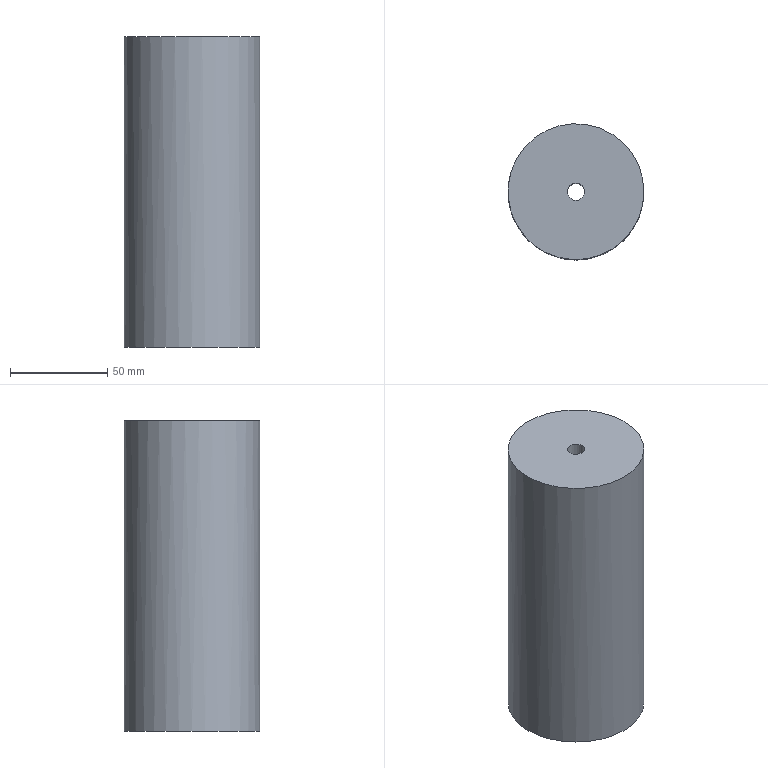Part | NX | features solid 2 | 1 solid | 4 faces | box 70 x 70 x 160 mm | volume 605573 mm3 | plane 2 | cylinder 2 | commonest cylinder face diameters 9 x1 70 x1
STEP:
#1=CARTESIAN_POINT('',(-1165.,525.,-35.));
#2=VERTEX_POINT('',#1);
#3=CARTESIAN_POINT('',(-1200.,525.,-35.));
#4=DIRECTION('',(0.,0.,-1.));
#5=DIRECTION('',(1.,0.,0.));
#6=AXIS2_PLACEMENT_3D('',#3,#4,#5);
#7=CIRCLE('',#6,35.);
#8=EDGE_CURVE('',#2,#2,#7,.F.);
#9=ORIENTED_EDGE('',*,*,#8,.T.);
#10=EDGE_LOOP('',(#9));
#11=FACE_BOUND('',#10,.T.);
#12=CARTESIAN_POINT('',(-1195.5,525.,-35.));
#13=VERTEX_POINT('',#12);
#14=CARTESIAN_POINT('',(-1200.,525.,-35.));
#15=DIRECTION('',(0.,0.,-1.));
#16=DIRECTION('',(1.,0.,0.));
#17=AXIS2_PLACEMENT_3D('',#14,#15,#16);
#18=CIRCLE('',#17,4.5);
#19=EDGE_CURVE('',#13,#13,#18,.T.);
#20=ORIENTED_EDGE('',*,*,#19,.T.);
#21=EDGE_LOOP('',(#20));
#22=FACE_BOUND('',#21,.T.);
#23=CARTESIAN_POINT('',(-1200.,525.,-35.));
#24=DIRECTION('',(0.,0.,1.));
#25=DIRECTION('',(-1.,0.,0.));
#26=AXIS2_PLACEMENT_3D('',#23,#24,#25);
#27=PLANE('',#26);
#28=ADVANCED_FACE('',(#11,#22),#27,.T.);
#29=CARTESIAN_POINT('',(-1235.,525.,-195.));
#30=VERTEX_POINT('',#29);
#31=CARTESIAN_POINT('',(-1200.,525.,-195.));
#32=DIRECTION('',(0.,0.,1.));
#33=DIRECTION('',(-1.,0.,0.));
#34=AXIS2_PLACEMENT_3D('',#31,#32,#33);
#35=CIRCLE('',#34,35.);
#36=EDGE_CURVE('',#30,#30,#35,.T.);
#37=ORIENTED_EDGE('',*,*,#36,.F.);
#38=EDGE_LOOP('',(#37));
#39=FACE_BOUND('',#38,.T.);
#40=CARTESIAN_POINT('',(-1204.5,525.,-195.));
#41=VERTEX_POINT('',#40);
#42=CARTESIAN_POINT('',(-1200.,525.,-195.));
#43=DIRECTION('',(0.,0.,1.));
#44=DIRECTION('',(-1.,0.,0.));
#45=AXIS2_PLACEMENT_3D('',#42,#43,#44);
#46=CIRCLE('',#45,4.5);
#47=EDGE_CURVE('',#41,#41,#46,.F.);
#48=ORIENTED_EDGE('',*,*,#47,.F.);
#49=EDGE_LOOP('',(#48));
#50=FACE_BOUND('',#49,.T.);
#51=CARTESIAN_POINT('',(-1200.,525.,-195.));
#52=DIRECTION('',(0.,0.,1.));
#53=DIRECTION('',(-1.,0.,0.));
#54=AXIS2_PLACEMENT_3D('',#51,#52,#53);
#55=PLANE('',#54);
#56=ADVANCED_FACE('',(#39,#50),#55,.F.);
#57=ORIENTED_EDGE('',*,*,#8,.F.);
#58=EDGE_LOOP('',(#57));
#59=FACE_BOUND('',#58,.T.);
#60=ORIENTED_EDGE('',*,*,#36,.T.);
#61=EDGE_LOOP('',(#60));
#62=FACE_BOUND('',#61,.T.);
#63=CARTESIAN_POINT('',(-1200.,525.,-100.));
#64=DIRECTION('',(0.,0.,-1.));
#65=DIRECTION('',(1.,0.,0.));
#66=AXIS2_PLACEMENT_3D('',#63,#64,#65);
#67=CYLINDRICAL_SURFACE('',#66,35.);
#68=ADVANCED_FACE('',(#59,#62),#67,.T.);
#69=ORIENTED_EDGE('',*,*,#19,.F.);
#70=EDGE_LOOP('',(#69));
#71=FACE_BOUND('',#70,.T.);
#72=ORIENTED_EDGE('',*,*,#47,.T.);
#73=EDGE_LOOP('',(#72));
#74=FACE_BOUND('',#73,.T.);
#75=CARTESIAN_POINT('',(-1200.,525.,-55.));
#76=DIRECTION('',(0.,0.,-1.));
#77=DIRECTION('',(1.,0.,0.));
#78=AXIS2_PLACEMENT_3D('',#75,#76,#77);
#79=CYLINDRICAL_SURFACE('',#78,4.5);
#80=ADVANCED_FACE('',(#71,#74),#79,.F.);
#81=CLOSED_SHELL('',(#28,#56,#68,#80));
#82=MANIFOLD_SOLID_BREP('',#81);
#83=(LENGTH_UNIT()NAMED_UNIT(*)SI_UNIT(.MILLI.,.METRE.));
#84=UNCERTAINTY_MEASURE_WITH_UNIT(LENGTH_MEASURE(0.00001),#83,'','');
#85=(NAMED_UNIT(*)PLANE_ANGLE_UNIT()SI_UNIT($,.RADIAN.));
#86=(NAMED_UNIT(*)SI_UNIT($,.STERADIAN.)SOLID_ANGLE_UNIT());
#87=(GEOMETRIC_REPRESENTATION_CONTEXT(3)GLOBAL_UNCERTAINTY_ASSIGNED_CONTEXT((#84))GLOBAL_UNIT_ASSIGNED_CONTEXT((#83,#85,#86))REPRESENTATION_CONTEXT('',''));
#88=ADVANCED_BREP_SHAPE_REPRESENTATION('',(#82),#87);